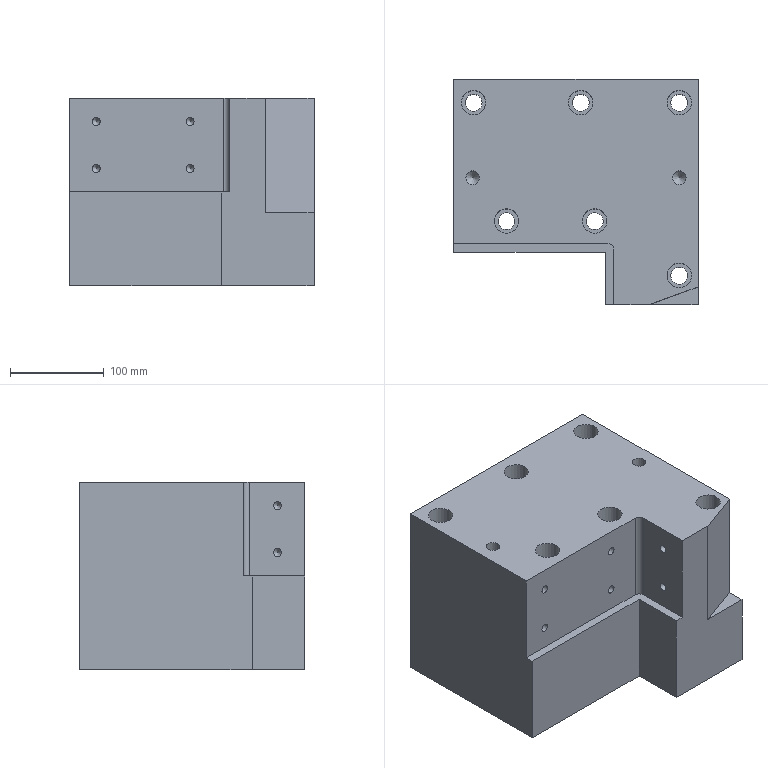Part | STEP file | lll_id4190_x_t | 1 solid | 48 faces | box 260 x 240 x 200 mm | volume 9818942 mm3 | cylinder 21 | plane 19 | cone 8 | commonest cylinder face diameters 8.506 x6 18.009 x6 26.008 x6 14.506 x2 12 x1
STEP:
#1=CARTESIAN_POINT('',(2885.753,309.047,34.253));
#2=VERTEX_POINT('',#1);
#3=CARTESIAN_POINT('',(2885.753,309.047,30.));
#4=DIRECTION('',(1.,0.,0.));
#5=DIRECTION('',(0.,0.,1.));
#6=AXIS2_PLACEMENT_3D('',#3,#4,#5);
#7=CIRCLE('',#6,4.253);
#8=EDGE_CURVE('',#2,#2,#7,.T.);
#9=ORIENTED_EDGE('',*,*,#8,.F.);
#10=EDGE_LOOP('',(#9));
#11=FACE_BOUND('',#10,.T.);
#12=CARTESIAN_POINT('',(2890.006,309.047,30.));
#13=VERTEX_POINT('',#12);
#14=VERTEX_LOOP('',#13);
#15=FACE_BOUND('',#14,.T.);
#16=CARTESIAN_POINT('',(2885.753,309.047,30.));
#17=DIRECTION('',(-1.,0.,0.));
#18=DIRECTION('',(0.,0.,-1.));
#19=AXIS2_PLACEMENT_3D('',#16,#17,#18);
#20=CONICAL_SURFACE('',#19,4.253,45.);
#21=ADVANCED_FACE('',(#11,#15),#20,.F.);
#22=CARTESIAN_POINT('',(2885.753,309.047,84.253));
#23=VERTEX_POINT('',#22);
#24=CARTESIAN_POINT('',(2885.753,309.047,80.));
#25=DIRECTION('',(1.,0.,0.));
#26=DIRECTION('',(0.,0.,1.));
#27=AXIS2_PLACEMENT_3D('',#24,#25,#26);
#28=CIRCLE('',#27,4.253);
#29=EDGE_CURVE('',#23,#23,#28,.T.);
#30=ORIENTED_EDGE('',*,*,#29,.F.);
#31=EDGE_LOOP('',(#30));
#32=FACE_BOUND('',#31,.T.);
#33=CARTESIAN_POINT('',(2890.006,309.047,80.));
#34=VERTEX_POINT('',#33);
#35=VERTEX_LOOP('',#34);
#36=FACE_BOUND('',#35,.T.);
#37=CARTESIAN_POINT('',(2885.753,309.047,80.));
#38=DIRECTION('',(-1.,0.,0.));
#39=DIRECTION('',(0.,0.,-1.));
#40=AXIS2_PLACEMENT_3D('',#37,#38,#39);
#41=CONICAL_SURFACE('',#40,4.253,45.);
#42=ADVANCED_FACE('',(#32,#36),#41,.F.);
#43=CARTESIAN_POINT('',(2703.,380.053,80.));
#44=VERTEX_POINT('',#43);
#45=VERTEX_LOOP('',#44);
#46=FACE_BOUND('',#45,.T.);
#47=CARTESIAN_POINT('',(2703.,375.8,75.747));
#48=VERTEX_POINT('',#47);
#49=CARTESIAN_POINT('',(2703.,375.8,80.));
#50=DIRECTION('',(0.,1.,0.));
#51=DIRECTION('',(0.,0.,-1.));
#52=AXIS2_PLACEMENT_3D('',#49,#50,#51);
#53=CIRCLE('',#52,4.253);
#54=EDGE_CURVE('',#48,#48,#53,.T.);
#55=ORIENTED_EDGE('',*,*,#54,.F.);
#56=EDGE_LOOP('',(#55));
#57=FACE_BOUND('',#56,.T.);
#58=CARTESIAN_POINT('',(2703.,375.8,80.));
#59=DIRECTION('',(0.,-1.,0.));
#60=DIRECTION('',(0.,0.,1.));
#61=AXIS2_PLACEMENT_3D('',#58,#59,#60);
#62=CONICAL_SURFACE('',#61,4.253,45.);
#63=ADVANCED_FACE('',(#46,#57),#62,.F.);
#64=CARTESIAN_POINT('',(2803.,380.053,80.));
#65=VERTEX_POINT('',#64);
#66=VERTEX_LOOP('',#65);
#67=FACE_BOUND('',#66,.T.);
#68=CARTESIAN_POINT('',(2803.,375.8,75.747));
#69=VERTEX_POINT('',#68);
#70=CARTESIAN_POINT('',(2803.,375.8,80.));
#71=DIRECTION('',(0.,1.,0.));
#72=DIRECTION('',(0.,0.,-1.));
#73=AXIS2_PLACEMENT_3D('',#70,#71,#72);
#74=CIRCLE('',#73,4.253);
#75=EDGE_CURVE('',#69,#69,#74,.T.);
#76=ORIENTED_EDGE('',*,*,#75,.F.);
#77=EDGE_LOOP('',(#76));
#78=FACE_BOUND('',#77,.T.);
#79=CARTESIAN_POINT('',(2803.,375.8,80.));
#80=DIRECTION('',(0.,-1.,0.));
#81=DIRECTION('',(0.,0.,1.));
#82=AXIS2_PLACEMENT_3D('',#79,#80,#81);
#83=CONICAL_SURFACE('',#82,4.253,45.);
#84=ADVANCED_FACE('',(#67,#78),#83,.F.);
#85=CARTESIAN_POINT('',(2703.,380.053,30.));
#86=VERTEX_POINT('',#85);
#87=VERTEX_LOOP('',#86);
#88=FACE_BOUND('',#87,.T.);
#89=CARTESIAN_POINT('',(2703.,375.8,25.747));
#90=VERTEX_POINT('',#89);
#91=CARTESIAN_POINT('',(2703.,375.8,30.));
#92=DIRECTION('',(0.,1.,0.));
#93=DIRECTION('',(0.,0.,-1.));
#94=AXIS2_PLACEMENT_3D('',#91,#92,#93);
#95=CIRCLE('',#94,4.253);
#96=EDGE_CURVE('',#90,#90,#95,.T.);
#97=ORIENTED_EDGE('',*,*,#96,.F.);
#98=EDGE_LOOP('',(#97));
#99=FACE_BOUND('',#98,.T.);
#100=CARTESIAN_POINT('',(2703.,375.8,30.));
#101=DIRECTION('',(0.,-1.,0.));
#102=DIRECTION('',(0.,0.,1.));
#103=AXIS2_PLACEMENT_3D('',#100,#101,#102);
#104=CONICAL_SURFACE('',#103,4.253,45.);
#105=ADVANCED_FACE('',(#88,#99),#104,.F.);
#106=CARTESIAN_POINT('',(2803.,380.053,30.));
#107=VERTEX_POINT('',#106);
#108=VERTEX_LOOP('',#107);
#109=FACE_BOUND('',#108,.T.);
#110=CARTESIAN_POINT('',(2803.,375.8,25.747));
#111=VERTEX_POINT('',#110);
#112=CARTESIAN_POINT('',(2803.,375.8,30.));
#113=DIRECTION('',(0.,1.,0.));
#114=DIRECTION('',(0.,0.,-1.));
#115=AXIS2_PLACEMENT_3D('',#112,#113,#114);
#116=CIRCLE('',#115,4.253);
#117=EDGE_CURVE('',#111,#111,#116,.T.);
#118=ORIENTED_EDGE('',*,*,#117,.F.);
#119=EDGE_LOOP('',(#118));
#120=FACE_BOUND('',#119,.T.);
#121=CARTESIAN_POINT('',(2803.,375.8,30.));
#122=DIRECTION('',(0.,-1.,0.));
#123=DIRECTION('',(0.,0.,1.));
#124=AXIS2_PLACEMENT_3D('',#121,#122,#123);
#125=CONICAL_SURFACE('',#124,4.253,45.);
#126=ADVANCED_FACE('',(#109,#120),#125,.F.);
#127=CARTESIAN_POINT('',(2924.005,495.047,-55.));
#128=VERTEX_POINT('',#127);
#129=CARTESIAN_POINT('',(2915.,495.047,-55.));
#130=DIRECTION('',(0.,0.,-1.));
#131=DIRECTION('',(1.,0.,0.));
#132=AXIS2_PLACEMENT_3D('',#129,#130,#131);
#133=CIRCLE('',#132,9.005);
#134=EDGE_CURVE('',#128,#128,#133,.T.);
#135=ORIENTED_EDGE('',*,*,#134,.T.);
#136=EDGE_LOOP('',(#135));
#137=FACE_BOUND('',#136,.T.);
#138=CARTESIAN_POINT('',(2901.996,495.047,-55.));
#139=VERTEX_POINT('',#138);
#140=CARTESIAN_POINT('',(2915.,495.047,-55.));
#141=DIRECTION('',(0.,0.,-1.));
#142=DIRECTION('',(-1.,0.,0.));
#143=AXIS2_PLACEMENT_3D('',#140,#141,#142);
#144=CIRCLE('',#143,13.004);
#145=EDGE_CURVE('',#139,#139,#144,.T.);
#146=ORIENTED_EDGE('',*,*,#145,.F.);
#147=EDGE_LOOP('',(#146));
#148=FACE_BOUND('',#147,.T.);
#149=CARTESIAN_POINT('',(2915.,495.047,-55.));
#150=DIRECTION('',(0.,0.,-1.));
#151=DIRECTION('',(1.,0.,0.));
#152=AXIS2_PLACEMENT_3D('',#149,#150,#151);
#153=PLANE('',#152);
#154=ADVANCED_FACE('',(#137,#148),#153,.F.);
#155=ORIENTED_EDGE('',*,*,#8,.T.);
#156=EDGE_LOOP('',(#155));
#157=FACE_BOUND('',#156,.T.);
#158=CARTESIAN_POINT('',(2845.,309.047,34.253));
#159=VERTEX_POINT('',#158);
#160=CARTESIAN_POINT('',(2845.,309.047,30.));
#161=DIRECTION('',(1.,0.,0.));
#162=DIRECTION('',(0.,0.,1.));
#163=AXIS2_PLACEMENT_3D('',#160,#161,#162);
#164=CIRCLE('',#163,4.253);
#165=EDGE_CURVE('',#159,#159,#164,.T.);
#166=ORIENTED_EDGE('',*,*,#165,.F.);
#167=EDGE_LOOP('',(#166));
#168=FACE_BOUND('',#167,.T.);
#169=CARTESIAN_POINT('',(2845.,309.047,30.));
#170=DIRECTION('',(1.,0.,0.));
#171=DIRECTION('',(0.,0.,1.));
#172=AXIS2_PLACEMENT_3D('',#169,#170,#171);
#173=CYLINDRICAL_SURFACE('',#172,4.253);
#174=ADVANCED_FACE('',(#157,#168),#173,.F.);
#175=ORIENTED_EDGE('',*,*,#29,.T.);
#176=EDGE_LOOP('',(#175));
#177=FACE_BOUND('',#176,.T.);
#178=CARTESIAN_POINT('',(2845.,309.047,84.253));
#179=VERTEX_POINT('',#178);
#180=CARTESIAN_POINT('',(2845.,309.047,80.));
#181=DIRECTION('',(1.,0.,0.));
#182=DIRECTION('',(0.,0.,1.));
#183=AXIS2_PLACEMENT_3D('',#180,#181,#182);
#184=CIRCLE('',#183,4.253);
#185=EDGE_CURVE('',#179,#179,#184,.T.);
#186=ORIENTED_EDGE('',*,*,#185,.F.);
#187=EDGE_LOOP('',(#186));
#188=FACE_BOUND('',#187,.T.);
#189=CARTESIAN_POINT('',(2845.,309.047,80.));
#190=DIRECTION('',(1.,0.,0.));
#191=DIRECTION('',(0.,0.,1.));
#192=AXIS2_PLACEMENT_3D('',#189,#190,#191);
#193=CYLINDRICAL_SURFACE('',#192,4.253);
#194=ADVANCED_FACE('',(#177,#188),#193,.F.);
#195=ORIENTED_EDGE('',*,*,#54,.T.);
#196=EDGE_LOOP('',(#195));
#197=FACE_BOUND('',#196,.T.);
#198=CARTESIAN_POINT('',(2698.747,345.047,80.));
#199=VERTEX_POINT('',#198);
#200=CARTESIAN_POINT('',(2703.,345.047,80.));
#201=DIRECTION('',(0.,1.,0.));
#202=DIRECTION('',(-1.,0.,0.));
#203=AXIS2_PLACEMENT_3D('',#200,#201,#202);
#204=CIRCLE('',#203,4.253);
#205=EDGE_CURVE('',#199,#199,#204,.T.);
#206=ORIENTED_EDGE('',*,*,#205,.F.);
#207=EDGE_LOOP('',(#206));
#208=FACE_BOUND('',#207,.T.);
#209=CARTESIAN_POINT('',(2703.,345.047,80.));
#210=DIRECTION('',(0.,1.,0.));
#211=DIRECTION('',(-1.,0.,0.));
#212=AXIS2_PLACEMENT_3D('',#209,#210,#211);
#213=CYLINDRICAL_SURFACE('',#212,4.253);
#214=ADVANCED_FACE('',(#197,#208),#213,.F.);
#215=ORIENTED_EDGE('',*,*,#75,.T.);
#216=EDGE_LOOP('',(#215));
#217=FACE_BOUND('',#216,.T.);
#218=CARTESIAN_POINT('',(2798.747,345.047,80.));
#219=VERTEX_POINT('',#218);
#220=CARTESIAN_POINT('',(2803.,345.047,80.));
#221=DIRECTION('',(0.,1.,0.));
#222=DIRECTION('',(-1.,0.,0.));
#223=AXIS2_PLACEMENT_3D('',#220,#221,#222);
#224=CIRCLE('',#223,4.253);
#225=EDGE_CURVE('',#219,#219,#224,.T.);
#226=ORIENTED_EDGE('',*,*,#225,.F.);
#227=EDGE_LOOP('',(#226));
#228=FACE_BOUND('',#227,.T.);
#229=CARTESIAN_POINT('',(2803.,345.047,80.));
#230=DIRECTION('',(0.,1.,0.));
#231=DIRECTION('',(-1.,0.,0.));
#232=AXIS2_PLACEMENT_3D('',#229,#230,#231);
#233=CYLINDRICAL_SURFACE('',#232,4.253);
#234=ADVANCED_FACE('',(#217,#228),#233,.F.);
#235=ORIENTED_EDGE('',*,*,#96,.T.);
#236=EDGE_LOOP('',(#235));
#237=FACE_BOUND('',#236,.T.);
#238=CARTESIAN_POINT('',(2698.747,345.047,30.));
#239=VERTEX_POINT('',#238);
#240=CARTESIAN_POINT('',(2703.,345.047,30.));
#241=DIRECTION('',(0.,1.,0.));
#242=DIRECTION('',(-1.,0.,0.));
#243=AXIS2_PLACEMENT_3D('',#240,#241,#242);
#244=CIRCLE('',#243,4.253);
#245=EDGE_CURVE('',#239,#239,#244,.T.);
#246=ORIENTED_EDGE('',*,*,#245,.F.);
#247=EDGE_LOOP('',(#246));
#248=FACE_BOUND('',#247,.T.);
#249=CARTESIAN_POINT('',(2703.,345.047,30.));
#250=DIRECTION('',(0.,1.,0.));
#251=DIRECTION('',(-1.,0.,0.));
#252=AXIS2_PLACEMENT_3D('',#249,#250,#251);
#253=CYLINDRICAL_SURFACE('',#252,4.253);
#254=ADVANCED_FACE('',(#237,#248),#253,.F.);
#255=ORIENTED_EDGE('',*,*,#117,.T.);
#256=EDGE_LOOP('',(#255));
#257=FACE_BOUND('',#256,.T.);
#258=CARTESIAN_POINT('',(2798.747,345.047,30.));
#259=VERTEX_POINT('',#258);
#260=CARTESIAN_POINT('',(2803.,345.047,30.));
#261=DIRECTION('',(0.,1.,0.));
#262=DIRECTION('',(-1.,0.,0.));
#263=AXIS2_PLACEMENT_3D('',#260,#261,#262);
#264=CIRCLE('',#263,4.253);
#265=EDGE_CURVE('',#259,#259,#264,.T.);
#266=ORIENTED_EDGE('',*,*,#265,.F.);
#267=EDGE_LOOP('',(#266));
#268=FACE_BOUND('',#267,.T.);
#269=CARTESIAN_POINT('',(2803.,345.047,30.));
#270=DIRECTION('',(0.,1.,0.));
#271=DIRECTION('',(-1.,0.,0.));
#272=AXIS2_PLACEMENT_3D('',#269,#270,#271);
#273=CYLINDRICAL_SURFACE('',#272,4.253);
#274=ADVANCED_FACE('',(#257,#268),#273,.F.);
#275=CARTESIAN_POINT('',(2845.,280.047,5.));
#276=VERTEX_POINT('',#275);
#277=CARTESIAN_POINT('',(2845.,339.047,5.));
#278=VERTEX_POINT('',#277);
#279=CARTESIAN_POINT('',(2845.,273.323,5.));
#280=DIRECTION('',(0.,1.,0.));
#281=VECTOR('',#280,1.);
#282=LINE('',#279,#281);
#283=EDGE_CURVE('',#276,#278,#282,.T.);
#284=ORIENTED_EDGE('',*,*,#283,.T.);
#285=CARTESIAN_POINT('',(2839.,345.047,5.));
#286=VERTEX_POINT('',#285);
#287=CARTESIAN_POINT('',(2839.,339.047,5.));
#288=DIRECTION('',(0.,0.,1.));
#289=DIRECTION('',(1.,0.,0.));
#290=AXIS2_PLACEMENT_3D('',#287,#288,#289);
#291=CIRCLE('',#290,6.);
#292=EDGE_CURVE('',#278,#286,#291,.T.);
#293=ORIENTED_EDGE('',*,*,#292,.T.);
#294=CARTESIAN_POINT('',(2675.,345.047,5.));
#295=VERTEX_POINT('',#294);
#296=CARTESIAN_POINT('',(2132.435,345.047,5.));
#297=DIRECTION('',(1.,0.,0.));
#298=VECTOR('',#297,1.);
#299=LINE('',#296,#298);
#300=EDGE_CURVE('',#295,#286,#299,.T.);
#301=ORIENTED_EDGE('',*,*,#300,.F.);
#302=CARTESIAN_POINT('',(2675.,336.047,5.));
#303=VERTEX_POINT('',#302);
#304=CARTESIAN_POINT('',(2675.,350.047,5.));
#305=DIRECTION('',(0.,1.,0.));
#306=VECTOR('',#305,1.);
#307=LINE('',#304,#306);
#308=EDGE_CURVE('',#303,#295,#307,.T.);
#309=ORIENTED_EDGE('',*,*,#308,.F.);
#310=CARTESIAN_POINT('',(2836.,336.047,5.));
#311=VERTEX_POINT('',#310);
#312=CARTESIAN_POINT('',(2132.435,336.047,5.));
#313=DIRECTION('',(-1.,0.,0.));
#314=VECTOR('',#313,1.);
#315=LINE('',#312,#314);
#316=EDGE_CURVE('',#311,#303,#315,.T.);
#317=ORIENTED_EDGE('',*,*,#316,.F.);
#318=CARTESIAN_POINT('',(2836.,280.047,5.));
#319=VERTEX_POINT('',#318);
#320=CARTESIAN_POINT('',(2836.,1.,5.));
#321=DIRECTION('',(0.,1.,0.));
#322=VECTOR('',#321,1.);
#323=LINE('',#320,#322);
#324=EDGE_CURVE('',#319,#311,#323,.T.);
#325=ORIENTED_EDGE('',*,*,#324,.F.);
#326=CARTESIAN_POINT('',(2132.435,280.047,5.));
#327=DIRECTION('',(1.,0.,0.));
#328=VECTOR('',#327,1.);
#329=LINE('',#326,#328);
#330=EDGE_CURVE('',#319,#276,#329,.T.);
#331=ORIENTED_EDGE('',*,*,#330,.T.);
#332=EDGE_LOOP('',(#284,#293,#301,#309,#317,#325,#331));
#333=FACE_OUTER_BOUND('',#332,.T.);
#334=CARTESIAN_POINT('',(2132.435,0.,5.));
#335=DIRECTION('',(0.,0.,1.));
#336=DIRECTION('',(1.,0.,0.));
#337=AXIS2_PLACEMENT_3D('',#334,#335,#336);
#338=PLANE('',#337);
#339=ADVANCED_FACE('',(#333),#338,.T.);
#340=CARTESIAN_POINT('',(2935.,280.047,-17.));
#341=VERTEX_POINT('',#340);
#342=CARTESIAN_POINT('',(2883.289,280.047,-17.));
#343=VERTEX_POINT('',#342);
#344=CARTESIAN_POINT('',(2655.,280.047,-17.));
#345=DIRECTION('',(-1.,0.,0.));
#346=VECTOR('',#345,1.);
#347=LINE('',#344,#346);
#348=EDGE_CURVE('',#341,#343,#347,.T.);
#349=ORIENTED_EDGE('',*,*,#348,.F.);
#350=CARTESIAN_POINT('',(2935.,298.868,-17.));
#351=VERTEX_POINT('',#350);
#352=CARTESIAN_POINT('',(2935.,365.047,-17.));
#353=DIRECTION('',(0.,-1.,0.));
#354=VECTOR('',#353,1.);
#355=LINE('',#352,#354);
#356=EDGE_CURVE('',#351,#341,#355,.T.);
#357=ORIENTED_EDGE('',*,*,#356,.F.);
#358=CARTESIAN_POINT('',(2927.313,296.07,-17.));
#359=DIRECTION('',(0.9397,0.342,0.));
#360=VECTOR('',#359,1.);
#361=LINE('',#358,#360);
#362=EDGE_CURVE('',#343,#351,#361,.T.);
#363=ORIENTED_EDGE('',*,*,#362,.F.);
#364=EDGE_LOOP('',(#349,#357,#363));
#365=FACE_OUTER_BOUND('',#364,.T.);
#366=CARTESIAN_POINT('',(2805.,365.047,-17.));
#367=DIRECTION('',(0.,0.,1.));
#368=DIRECTION('',(1.,0.,0.));
#369=AXIS2_PLACEMENT_3D('',#366,#367,#368);
#370=PLANE('',#369);
#371=ADVANCED_FACE('',(#365),#370,.T.);
#372=CARTESIAN_POINT('',(2695.,415.047,61.994));
#373=VERTEX_POINT('',#372);
#374=VERTEX_LOOP('',#373);
#375=FACE_BOUND('',#374,.T.);
#376=CARTESIAN_POINT('',(2702.253,415.047,69.247));
#377=VERTEX_POINT('',#376);
#378=CARTESIAN_POINT('',(2695.,415.047,69.247));
#379=DIRECTION('',(0.,0.,-1.));
#380=DIRECTION('',(1.,0.,0.));
#381=AXIS2_PLACEMENT_3D('',#378,#379,#380);
#382=CIRCLE('',#381,7.253);
#383=EDGE_CURVE('',#377,#377,#382,.T.);
#384=ORIENTED_EDGE('',*,*,#383,.F.);
#385=EDGE_LOOP('',(#384));
#386=FACE_BOUND('',#385,.T.);
#387=CARTESIAN_POINT('',(2695.,415.047,69.247));
#388=DIRECTION('',(0.,0.,1.));
#389=DIRECTION('',(-1.,0.,0.));
#390=AXIS2_PLACEMENT_3D('',#387,#388,#389);
#391=CONICAL_SURFACE('',#390,7.253,45.);
#392=ADVANCED_FACE('',(#375,#386),#391,.F.);
#393=CARTESIAN_POINT('',(2915.,415.047,61.994));
#394=VERTEX_POINT('',#393);
#395=VERTEX_LOOP('',#394);
#396=FACE_BOUND('',#395,.T.);
#397=CARTESIAN_POINT('',(2907.747,415.047,69.247));
#398=VERTEX_POINT('',#397);
#399=CARTESIAN_POINT('',(2915.,415.047,69.247));
#400=DIRECTION('',(0.,0.,-1.));
#401=DIRECTION('',(-1.,0.,0.));
#402=AXIS2_PLACEMENT_3D('',#399,#400,#401);
#403=CIRCLE('',#402,7.253);
#404=EDGE_CURVE('',#398,#398,#403,.T.);
#405=ORIENTED_EDGE('',*,*,#404,.F.);
#406=EDGE_LOOP('',(#405));
#407=FACE_BOUND('',#406,.T.);
#408=CARTESIAN_POINT('',(2915.,415.047,69.247));
#409=DIRECTION('',(0.,0.,1.));
#410=DIRECTION('',(1.,0.,0.));
#411=AXIS2_PLACEMENT_3D('',#408,#409,#410);
#412=CONICAL_SURFACE('',#411,7.253,45.);
#413=ADVANCED_FACE('',(#396,#407),#412,.F.);
#414=CARTESIAN_POINT('',(2924.005,311.047,-55.));
#415=VERTEX_POINT('',#414);
#416=CARTESIAN_POINT('',(2915.,311.047,-55.));
#417=DIRECTION('',(0.,0.,-1.));
#418=DIRECTION('',(1.,0.,0.));
#419=AXIS2_PLACEMENT_3D('',#416,#417,#418);
#420=CIRCLE('',#419,9.005);
#421=EDGE_CURVE('',#415,#415,#420,.T.);
#422=ORIENTED_EDGE('',*,*,#421,.T.);
#423=EDGE_LOOP('',(#422));
#424=FACE_BOUND('',#423,.T.);
#425=CARTESIAN_POINT('',(2901.996,311.047,-55.));
#426=VERTEX_POINT('',#425);
#427=CARTESIAN_POINT('',(2915.,311.047,-55.));
#428=DIRECTION('',(0.,0.,-1.));
#429=DIRECTION('',(-1.,0.,0.));
#430=AXIS2_PLACEMENT_3D('',#427,#428,#429);
#431=CIRCLE('',#430,13.004);
#432=EDGE_CURVE('',#426,#426,#431,.T.);
#433=ORIENTED_EDGE('',*,*,#432,.F.);
#434=EDGE_LOOP('',(#433));
#435=FACE_BOUND('',#434,.T.);
#436=CARTESIAN_POINT('',(2915.,311.047,-55.));
#437=DIRECTION('',(0.,0.,-1.));
#438=DIRECTION('',(1.,0.,0.));
#439=AXIS2_PLACEMENT_3D('',#436,#437,#438);
#440=PLANE('',#439);
#441=ADVANCED_FACE('',(#424,#435),#440,.F.);
#442=CARTESIAN_POINT('',(2819.005,495.047,-55.));
#443=VERTEX_POINT('',#442);
#444=CARTESIAN_POINT('',(2810.,495.047,-55.));
#445=DIRECTION('',(0.,0.,-1.));
#446=DIRECTION('',(1.,0.,0.));
#447=AXIS2_PLACEMENT_3D('',#444,#445,#446);
#448=CIRCLE('',#447,9.005);
#449=EDGE_CURVE('',#443,#443,#448,.T.);
#450=ORIENTED_EDGE('',*,*,#449,.T.);
#451=EDGE_LOOP('',(#450));
#452=FACE_BOUND('',#451,.T.);
#453=CARTESIAN_POINT('',(2796.996,495.047,-55.));
#454=VERTEX_POINT('',#453);
#455=CARTESIAN_POINT('',(2810.,495.047,-55.));
#456=DIRECTION('',(0.,0.,-1.));
#457=DIRECTION('',(-1.,0.,0.));
#458=AXIS2_PLACEMENT_3D('',#455,#456,#457);
#459=CIRCLE('',#458,13.004);
#460=EDGE_CURVE('',#454,#454,#459,.T.);
#461=ORIENTED_EDGE('',*,*,#460,.F.);
#462=EDGE_LOOP('',(#461));
#463=FACE_BOUND('',#462,.T.);
#464=CARTESIAN_POINT('',(2810.,495.047,-55.));
#465=DIRECTION('',(0.,0.,-1.));
#466=DIRECTION('',(1.,0.,0.));
#467=AXIS2_PLACEMENT_3D('',#464,#465,#466);
#468=PLANE('',#467);
#469=ADVANCED_FACE('',(#452,#463),#468,.F.);
#470=CARTESIAN_POINT('',(2705.005,495.047,-55.));
#471=VERTEX_POINT('',#470);
#472=CARTESIAN_POINT('',(2696.,495.047,-55.));
#473=DIRECTION('',(0.,0.,-1.));
#474=DIRECTION('',(1.,0.,0.));
#475=AXIS2_PLACEMENT_3D('',#472,#473,#474);
#476=CIRCLE('',#475,9.005);
#477=EDGE_CURVE('',#471,#471,#476,.T.);
#478=ORIENTED_EDGE('',*,*,#477,.T.);
#479=EDGE_LOOP('',(#478));
#480=FACE_BOUND('',#479,.T.);
#481=CARTESIAN_POINT('',(2682.996,495.047,-55.));
#482=VERTEX_POINT('',#481);
#483=CARTESIAN_POINT('',(2696.,495.047,-55.));
#484=DIRECTION('',(0.,0.,-1.));
#485=DIRECTION('',(-1.,0.,0.));
#486=AXIS2_PLACEMENT_3D('',#483,#484,#485);
#487=CIRCLE('',#486,13.004);
#488=EDGE_CURVE('',#482,#482,#487,.T.);
#489=ORIENTED_EDGE('',*,*,#488,.F.);
#490=EDGE_LOOP('',(#489));
#491=FACE_BOUND('',#490,.T.);
#492=CARTESIAN_POINT('',(2696.,495.047,-55.));
#493=DIRECTION('',(0.,0.,-1.));
#494=DIRECTION('',(1.,0.,0.));
#495=AXIS2_PLACEMENT_3D('',#492,#493,#494);
#496=PLANE('',#495);
#497=ADVANCED_FACE('',(#480,#491),#496,.F.);
#498=CARTESIAN_POINT('',(2834.005,369.047,-55.));
#499=VERTEX_POINT('',#498);
#500=CARTESIAN_POINT('',(2825.,369.047,-55.));
#501=DIRECTION('',(0.,0.,-1.));
#502=DIRECTION('',(1.,0.,0.));
#503=AXIS2_PLACEMENT_3D('',#500,#501,#502);
#504=CIRCLE('',#503,9.005);
#505=EDGE_CURVE('',#499,#499,#504,.T.);
#506=ORIENTED_EDGE('',*,*,#505,.T.);
#507=EDGE_LOOP('',(#506));
#508=FACE_BOUND('',#507,.T.);
#509=CARTESIAN_POINT('',(2811.996,369.047,-55.));
#510=VERTEX_POINT('',#509);
#511=CARTESIAN_POINT('',(2825.,369.047,-55.));
#512=DIRECTION('',(0.,0.,-1.));
#513=DIRECTION('',(-1.,0.,0.));
#514=AXIS2_PLACEMENT_3D('',#511,#512,#513);
#515=CIRCLE('',#514,13.004);
#516=EDGE_CURVE('',#510,#510,#515,.T.);
#517=ORIENTED_EDGE('',*,*,#516,.F.);
#518=EDGE_LOOP('',(#517));
#519=FACE_BOUND('',#518,.T.);
#520=CARTESIAN_POINT('',(2825.,369.047,-55.));
#521=DIRECTION('',(0.,0.,-1.));
#522=DIRECTION('',(1.,0.,0.));
#523=AXIS2_PLACEMENT_3D('',#520,#521,#522);
#524=PLANE('',#523);
#525=ADVANCED_FACE('',(#508,#519),#524,.F.);
#526=CARTESIAN_POINT('',(2675.,336.047,-95.));
#527=VERTEX_POINT('',#526);
#528=CARTESIAN_POINT('',(2675.,336.047,-65.));
#529=DIRECTION('',(0.,0.,-1.));
#530=VECTOR('',#529,1.);
#531=LINE('',#528,#530);
#532=EDGE_CURVE('',#303,#527,#531,.T.);
#533=ORIENTED_EDGE('',*,*,#532,.T.);
#534=CARTESIAN_POINT('',(2836.,336.047,-95.));
#535=VERTEX_POINT('',#534);
#536=CARTESIAN_POINT('',(2655.,336.047,-95.));
#537=DIRECTION('',(-1.,0.,0.));
#538=VECTOR('',#537,1.);
#539=LINE('',#536,#538);
#540=EDGE_CURVE('',#535,#527,#539,.T.);
#541=ORIENTED_EDGE('',*,*,#540,.F.);
#542=CARTESIAN_POINT('',(2836.,336.047,-650.));
#543=DIRECTION('',(0.,0.,-1.));
#544=VECTOR('',#543,1.);
#545=LINE('',#542,#544);
#546=EDGE_CURVE('',#311,#535,#545,.T.);
#547=ORIENTED_EDGE('',*,*,#546,.F.);
#548=ORIENTED_EDGE('',*,*,#316,.T.);
#549=EDGE_LOOP('',(#533,#541,#547,#548));
#550=FACE_OUTER_BOUND('',#549,.T.);
#551=CARTESIAN_POINT('',(-2196.249,336.047,-650.));
#552=DIRECTION('',(0.,-1.,0.));
#553=DIRECTION('',(0.,0.,1.));
#554=AXIS2_PLACEMENT_3D('',#551,#552,#553);
#555=PLANE('',#554);
#556=ADVANCED_FACE('',(#550),#555,.T.);
#557=ORIENTED_EDGE('',*,*,#546,.T.);
#558=CARTESIAN_POINT('',(2836.,280.047,-95.));
#559=VERTEX_POINT('',#558);
#560=CARTESIAN_POINT('',(2836.,1.,-95.));
#561=DIRECTION('',(0.,1.,0.));
#562=VECTOR('',#561,1.);
#563=LINE('',#560,#562);
#564=EDGE_CURVE('',#559,#535,#563,.T.);
#565=ORIENTED_EDGE('',*,*,#564,.F.);
#566=CARTESIAN_POINT('',(2836.,280.047,-650.));
#567=DIRECTION('',(0.,0.,1.));
#568=VECTOR('',#567,1.);
#569=LINE('',#566,#568);
#570=EDGE_CURVE('',#559,#319,#569,.T.);
#571=ORIENTED_EDGE('',*,*,#570,.T.);
#572=ORIENTED_EDGE('',*,*,#324,.T.);
#573=EDGE_LOOP('',(#557,#565,#571,#572));
#574=FACE_OUTER_BOUND('',#573,.T.);
#575=CARTESIAN_POINT('',(2836.,1.,-650.));
#576=DIRECTION('',(1.,0.,0.));
#577=DIRECTION('',(0.,0.,1.));
#578=AXIS2_PLACEMENT_3D('',#575,#576,#577);
#579=PLANE('',#578);
#580=ADVANCED_FACE('',(#574),#579,.F.);
#581=CARTESIAN_POINT('',(2924.005,495.047,-95.));
#582=VERTEX_POINT('',#581);
#583=CARTESIAN_POINT('',(2915.,495.047,-95.));
#584=DIRECTION('',(0.,0.,-1.));
#585=DIRECTION('',(1.,0.,0.));
#586=AXIS2_PLACEMENT_3D('',#583,#584,#585);
#587=CIRCLE('',#586,9.005);
#588=EDGE_CURVE('',#582,#582,#587,.T.);
#589=ORIENTED_EDGE('',*,*,#588,.T.);
#590=EDGE_LOOP('',(#589));
#591=FACE_BOUND('',#590,.T.);
#592=ORIENTED_EDGE('',*,*,#134,.F.);
#593=EDGE_LOOP('',(#592));
#594=FACE_BOUND('',#593,.T.);
#595=CARTESIAN_POINT('',(2915.,495.047,107.));
#596=DIRECTION('',(0.,0.,-1.));
#597=DIRECTION('',(-1.,0.,0.));
#598=AXIS2_PLACEMENT_3D('',#595,#596,#597);
#599=CYLINDRICAL_SURFACE('',#598,9.005);
#600=ADVANCED_FACE('',(#591,#594),#599,.F.);
#601=ORIENTED_EDGE('',*,*,#145,.T.);
#602=EDGE_LOOP('',(#601));
#603=FACE_BOUND('',#602,.T.);
#604=CARTESIAN_POINT('',(2901.996,495.047,105.));
#605=VERTEX_POINT('',#604);
#606=CARTESIAN_POINT('',(2915.,495.047,105.));
#607=DIRECTION('',(0.,0.,-1.));
#608=DIRECTION('',(-1.,0.,0.));
#609=AXIS2_PLACEMENT_3D('',#606,#607,#608);
#610=CIRCLE('',#609,13.004);
#611=EDGE_CURVE('',#605,#605,#610,.T.);
#612=ORIENTED_EDGE('',*,*,#611,.F.);
#613=EDGE_LOOP('',(#612));
#614=FACE_BOUND('',#613,.T.);
#615=CARTESIAN_POINT('',(2915.,495.047,105.));
#616=DIRECTION('',(0.,0.,-1.));
#617=DIRECTION('',(-1.,0.,0.));
#618=AXIS2_PLACEMENT_3D('',#615,#616,#617);
#619=CYLINDRICAL_SURFACE('',#618,13.004);
#620=ADVANCED_FACE('',(#603,#614),#619,.F.);
#621=ORIENTED_EDGE('',*,*,#362,.T.);
#622=CARTESIAN_POINT('',(2935.,298.868,105.));
#623=VERTEX_POINT('',#622);
#624=CARTESIAN_POINT('',(2935.,298.868,-80.));
#625=DIRECTION('',(0.,0.,1.));
#626=VECTOR('',#625,1.);
#627=LINE('',#624,#626);
#628=EDGE_CURVE('',#351,#623,#627,.T.);
#629=ORIENTED_EDGE('',*,*,#628,.T.);
#630=CARTESIAN_POINT('',(2883.289,280.047,105.));
#631=VERTEX_POINT('',#630);
#632=CARTESIAN_POINT('',(2677.687,205.214,105.));
#633=DIRECTION('',(-0.9397,-0.342,0.));
#634=VECTOR('',#633,1.);
#635=LINE('',#632,#634);
#636=EDGE_CURVE('',#623,#631,#635,.T.);
#637=ORIENTED_EDGE('',*,*,#636,.T.);
#638=CARTESIAN_POINT('',(2883.289,280.047,-80.));
#639=DIRECTION('',(0.,0.,-1.));
#640=VECTOR('',#639,1.);
#641=LINE('',#638,#640);
#642=EDGE_CURVE('',#631,#343,#641,.T.);
#643=ORIENTED_EDGE('',*,*,#642,.T.);
#644=EDGE_LOOP('',(#621,#629,#637,#643));
#645=FACE_OUTER_BOUND('',#644,.T.);
#646=CARTESIAN_POINT('',(2927.313,296.07,-80.));
#647=DIRECTION('',(0.342,-0.9397,0.));
#648=DIRECTION('',(0.,0.,-1.));
#649=AXIS2_PLACEMENT_3D('',#646,#647,#648);
#650=PLANE('',#649);
#651=ADVANCED_FACE('',(#645),#650,.T.);
#652=ORIENTED_EDGE('',*,*,#348,.T.);
#653=ORIENTED_EDGE('',*,*,#642,.F.);
#654=CARTESIAN_POINT('',(2845.,280.047,105.));
#655=VERTEX_POINT('',#654);
#656=CARTESIAN_POINT('',(2655.,280.047,105.));
#657=DIRECTION('',(-1.,0.,0.));
#658=VECTOR('',#657,1.);
#659=LINE('',#656,#658);
#660=EDGE_CURVE('',#631,#655,#659,.T.);
#661=ORIENTED_EDGE('',*,*,#660,.T.);
#662=CARTESIAN_POINT('',(2845.,280.047,171.231));
#663=DIRECTION('',(0.,0.,1.));
#664=VECTOR('',#663,1.);
#665=LINE('',#662,#664);
#666=EDGE_CURVE('',#276,#655,#665,.T.);
#667=ORIENTED_EDGE('',*,*,#666,.F.);
#668=ORIENTED_EDGE('',*,*,#330,.F.);
#669=ORIENTED_EDGE('',*,*,#570,.F.);
#670=CARTESIAN_POINT('',(2935.,280.047,-95.));
#671=VERTEX_POINT('',#670);
#672=CARTESIAN_POINT('',(2655.,280.047,-95.));
#673=DIRECTION('',(-1.,0.,0.));
#674=VECTOR('',#673,1.);
#675=LINE('',#672,#674);
#676=EDGE_CURVE('',#671,#559,#675,.T.);
#677=ORIENTED_EDGE('',*,*,#676,.F.);
#678=CARTESIAN_POINT('',(2935.,280.047,-65.));
#679=DIRECTION('',(0.,0.,-1.));
#680=VECTOR('',#679,1.);
#681=LINE('',#678,#680);
#682=EDGE_CURVE('',#341,#671,#681,.T.);
#683=ORIENTED_EDGE('',*,*,#682,.F.);
#684=EDGE_LOOP('',(#652,#653,#661,#667,#668,#669,#677,#683));
#685=FACE_OUTER_BOUND('',#684,.T.);
#686=CARTESIAN_POINT('',(2655.,280.047,-65.));
#687=DIRECTION('',(0.,1.,0.));
#688=DIRECTION('',(0.,0.,-1.));
#689=AXIS2_PLACEMENT_3D('',#686,#687,#688);
#690=PLANE('',#689);
#691=ADVANCED_FACE('',(#685),#690,.F.);
#692=ORIENTED_EDGE('',*,*,#185,.T.);
#693=EDGE_LOOP('',(#692));
#694=FACE_BOUND('',#693,.T.);
#695=ORIENTED_EDGE('',*,*,#165,.T.);
#696=EDGE_LOOP('',(#695));
#697=FACE_BOUND('',#696,.T.);
#698=CARTESIAN_POINT('',(2845.,339.047,105.));
#699=VERTEX_POINT('',#698);
#700=CARTESIAN_POINT('',(2845.,267.547,105.));
#701=DIRECTION('',(0.,1.,0.));
#702=VECTOR('',#701,1.);
#703=LINE('',#700,#702);
#704=EDGE_CURVE('',#655,#699,#703,.T.);
#705=ORIENTED_EDGE('',*,*,#704,.T.);
#706=CARTESIAN_POINT('',(2845.,339.047,5.));
#707=DIRECTION('',(0.,0.,-1.));
#708=VECTOR('',#707,1.);
#709=LINE('',#706,#708);
#710=EDGE_CURVE('',#699,#278,#709,.T.);
#711=ORIENTED_EDGE('',*,*,#710,.T.);
#712=ORIENTED_EDGE('',*,*,#283,.F.);
#713=ORIENTED_EDGE('',*,*,#666,.T.);
#714=EDGE_LOOP('',(#705,#711,#712,#713));
#715=FACE_BOUND('',#714,.T.);
#716=CARTESIAN_POINT('',(2845.,273.323,171.231));
#717=DIRECTION('',(1.,0.,0.));
#718=DIRECTION('',(0.,0.,1.));
#719=AXIS2_PLACEMENT_3D('',#716,#717,#718);
#720=PLANE('',#719);
#721=ADVANCED_FACE('',(#694,#697,#715),#720,.F.);
#722=ORIENTED_EDGE('',*,*,#265,.T.);
#723=EDGE_LOOP('',(#722));
#724=FACE_BOUND('',#723,.T.);
#725=ORIENTED_EDGE('',*,*,#245,.T.);
#726=EDGE_LOOP('',(#725));
#727=FACE_BOUND('',#726,.T.);
#728=ORIENTED_EDGE('',*,*,#225,.T.);
#729=EDGE_LOOP('',(#728));
#730=FACE_BOUND('',#729,.T.);
#731=ORIENTED_EDGE('',*,*,#205,.T.);
#732=EDGE_LOOP('',(#731));
#733=FACE_BOUND('',#732,.T.);
#734=ORIENTED_EDGE('',*,*,#300,.T.);
#735=CARTESIAN_POINT('',(2839.,345.047,105.));
#736=VERTEX_POINT('',#735);
#737=CARTESIAN_POINT('',(2839.,345.047,105.));
#738=DIRECTION('',(0.,0.,1.));
#739=VECTOR('',#738,1.);
#740=LINE('',#737,#739);
#741=EDGE_CURVE('',#286,#736,#740,.T.);
#742=ORIENTED_EDGE('',*,*,#741,.T.);
#743=CARTESIAN_POINT('',(2675.,345.047,105.));
#744=VERTEX_POINT('',#743);
#745=CARTESIAN_POINT('',(2655.,345.047,105.));
#746=DIRECTION('',(-1.,0.,0.));
#747=VECTOR('',#746,1.);
#748=LINE('',#745,#747);
#749=EDGE_CURVE('',#736,#744,#748,.T.);
#750=ORIENTED_EDGE('',*,*,#749,.T.);
#751=CARTESIAN_POINT('',(2675.,345.047,170.851));
#752=DIRECTION('',(0.,0.,-1.));
#753=VECTOR('',#752,1.);
#754=LINE('',#751,#753);
#755=EDGE_CURVE('',#744,#295,#754,.T.);
#756=ORIENTED_EDGE('',*,*,#755,.T.);
#757=EDGE_LOOP('',(#734,#742,#750,#756));
#758=FACE_BOUND('',#757,.T.);
#759=CARTESIAN_POINT('',(2685.,345.047,170.851));
#760=DIRECTION('',(0.,1.,0.));
#761=DIRECTION('',(0.,0.,-1.));
#762=AXIS2_PLACEMENT_3D('',#759,#760,#761);
#763=PLANE('',#762);
#764=ADVANCED_FACE('',(#724,#727,#730,#733,#758),#763,.F.);
#765=CARTESIAN_POINT('',(2675.,520.047,-95.));
#766=VERTEX_POINT('',#765);
#767=CARTESIAN_POINT('',(2675.,520.047,105.));
#768=VERTEX_POINT('',#767);
#769=CARTESIAN_POINT('',(2675.,520.047,-65.));
#770=DIRECTION('',(0.,0.,1.));
#771=VECTOR('',#770,1.);
#772=LINE('',#769,#771);
#773=EDGE_CURVE('',#766,#768,#772,.T.);
#774=ORIENTED_EDGE('',*,*,#773,.F.);
#775=CARTESIAN_POINT('',(2675.,350.047,-95.));
#776=DIRECTION('',(0.,1.,0.));
#777=VECTOR('',#776,1.);
#778=LINE('',#775,#777);
#779=EDGE_CURVE('',#527,#766,#778,.T.);
#780=ORIENTED_EDGE('',*,*,#779,.F.);
#781=ORIENTED_EDGE('',*,*,#532,.F.);
#782=ORIENTED_EDGE('',*,*,#308,.T.);
#783=ORIENTED_EDGE('',*,*,#755,.F.);
#784=CARTESIAN_POINT('',(2675.,267.547,105.));
#785=DIRECTION('',(0.,1.,0.));
#786=VECTOR('',#785,1.);
#787=LINE('',#784,#786);
#788=EDGE_CURVE('',#744,#768,#787,.T.);
#789=ORIENTED_EDGE('',*,*,#788,.T.);
#790=EDGE_LOOP('',(#774,#780,#781,#782,#783,#789));
#791=FACE_OUTER_BOUND('',#790,.T.);
#792=CARTESIAN_POINT('',(2675.,350.047,-65.));
#793=DIRECTION('',(1.,0.,0.));
#794=DIRECTION('',(0.,0.,1.));
#795=AXIS2_PLACEMENT_3D('',#792,#793,#794);
#796=PLANE('',#795);
#797=ADVANCED_FACE('',(#791),#796,.F.);
#798=CARTESIAN_POINT('',(2935.,520.047,-95.));
#799=VERTEX_POINT('',#798);
#800=CARTESIAN_POINT('',(2935.,520.047,105.));
#801=VERTEX_POINT('',#800);
#802=CARTESIAN_POINT('',(2935.,520.047,-80.));
#803=DIRECTION('',(0.,0.,1.));
#804=VECTOR('',#803,1.);
#805=LINE('',#802,#804);
#806=EDGE_CURVE('',#799,#801,#805,.T.);
#807=ORIENTED_EDGE('',*,*,#806,.F.);
#808=CARTESIAN_POINT('',(2655.,520.047,-95.));
#809=DIRECTION('',(-1.,0.,0.));
#810=VECTOR('',#809,1.);
#811=LINE('',#808,#810);
#812=EDGE_CURVE('',#799,#766,#811,.T.);
#813=ORIENTED_EDGE('',*,*,#812,.T.);
#814=ORIENTED_EDGE('',*,*,#773,.T.);
#815=CARTESIAN_POINT('',(2655.,520.047,105.));
#816=DIRECTION('',(1.,0.,0.));
#817=VECTOR('',#816,1.);
#818=LINE('',#815,#817);
#819=EDGE_CURVE('',#768,#801,#818,.T.);
#820=ORIENTED_EDGE('',*,*,#819,.T.);
#821=EDGE_LOOP('',(#807,#813,#814,#820));
#822=FACE_OUTER_BOUND('',#821,.T.);
#823=CARTESIAN_POINT('',(2655.,520.047,-80.));
#824=DIRECTION('',(0.,1.,0.));
#825=DIRECTION('',(0.,0.,-1.));
#826=AXIS2_PLACEMENT_3D('',#823,#824,#825);
#827=PLANE('',#826);
#828=ADVANCED_FACE('',(#822),#827,.T.);
#829=ORIENTED_EDGE('',*,*,#356,.T.);
#830=ORIENTED_EDGE('',*,*,#682,.T.);
#831=CARTESIAN_POINT('',(2935.,267.547,-95.));
#832=DIRECTION('',(0.,1.,0.));
#833=VECTOR('',#832,1.);
#834=LINE('',#831,#833);
#835=EDGE_CURVE('',#671,#799,#834,.T.);
#836=ORIENTED_EDGE('',*,*,#835,.T.);
#837=ORIENTED_EDGE('',*,*,#806,.T.);
#838=CARTESIAN_POINT('',(2935.,267.547,105.));
#839=DIRECTION('',(0.,-1.,0.));
#840=VECTOR('',#839,1.);
#841=LINE('',#838,#840);
#842=EDGE_CURVE('',#801,#623,#841,.T.);
#843=ORIENTED_EDGE('',*,*,#842,.T.);
#844=ORIENTED_EDGE('',*,*,#628,.F.);
#845=EDGE_LOOP('',(#829,#830,#836,#837,#843,#844));
#846=FACE_OUTER_BOUND('',#845,.T.);
#847=CARTESIAN_POINT('',(2935.,267.547,-80.));
#848=DIRECTION('',(1.,0.,0.));
#849=DIRECTION('',(0.,0.,1.));
#850=AXIS2_PLACEMENT_3D('',#847,#848,#849);
#851=PLANE('',#850);
#852=ADVANCED_FACE('',(#846),#851,.T.);
#853=CARTESIAN_POINT('',(2687.747,415.047,105.));
#854=VERTEX_POINT('',#853);
#855=CARTESIAN_POINT('',(2695.,415.047,105.));
#856=DIRECTION('',(0.,0.,1.));
#857=DIRECTION('',(-1.,0.,0.));
#858=AXIS2_PLACEMENT_3D('',#855,#856,#857);
#859=CIRCLE('',#858,7.253);
#860=EDGE_CURVE('',#854,#854,#859,.T.);
#861=ORIENTED_EDGE('',*,*,#860,.T.);
#862=EDGE_LOOP('',(#861));
#863=FACE_BOUND('',#862,.T.);
#864=ORIENTED_EDGE('',*,*,#383,.T.);
#865=EDGE_LOOP('',(#864));
#866=FACE_BOUND('',#865,.T.);
#867=CARTESIAN_POINT('',(2695.,415.047,107.));
#868=DIRECTION('',(0.,0.,-1.));
#869=DIRECTION('',(-1.,0.,0.));
#870=AXIS2_PLACEMENT_3D('',#867,#868,#869);
#871=CYLINDRICAL_SURFACE('',#870,7.253);
#872=ADVANCED_FACE('',(#863,#866),#871,.F.);
#873=CARTESIAN_POINT('',(2922.253,415.047,105.));
#874=VERTEX_POINT('',#873);
#875=CARTESIAN_POINT('',(2915.,415.047,105.));
#876=DIRECTION('',(0.,0.,1.));
#877=DIRECTION('',(1.,0.,0.));
#878=AXIS2_PLACEMENT_3D('',#875,#876,#877);
#879=CIRCLE('',#878,7.253);
#880=EDGE_CURVE('',#874,#874,#879,.T.);
#881=ORIENTED_EDGE('',*,*,#880,.T.);
#882=EDGE_LOOP('',(#881));
#883=FACE_BOUND('',#882,.T.);
#884=ORIENTED_EDGE('',*,*,#404,.T.);
#885=EDGE_LOOP('',(#884));
#886=FACE_BOUND('',#885,.T.);
#887=CARTESIAN_POINT('',(2915.,415.047,107.));
#888=DIRECTION('',(0.,0.,-1.));
#889=DIRECTION('',(1.,0.,0.));
#890=AXIS2_PLACEMENT_3D('',#887,#888,#889);
#891=CYLINDRICAL_SURFACE('',#890,7.253);
#892=ADVANCED_FACE('',(#883,#886),#891,.F.);
#893=ORIENTED_EDGE('',*,*,#432,.T.);
#894=EDGE_LOOP('',(#893));
#895=FACE_BOUND('',#894,.T.);
#896=CARTESIAN_POINT('',(2928.004,311.047,105.));
#897=VERTEX_POINT('',#896);
#898=CARTESIAN_POINT('',(2915.,311.047,105.));
#899=DIRECTION('',(0.,0.,1.));
#900=DIRECTION('',(1.,0.,0.));
#901=AXIS2_PLACEMENT_3D('',#898,#899,#900);
#902=CIRCLE('',#901,13.004);
#903=EDGE_CURVE('',#897,#897,#902,.T.);
#904=ORIENTED_EDGE('',*,*,#903,.T.);
#905=EDGE_LOOP('',(#904));
#906=FACE_BOUND('',#905,.T.);
#907=CARTESIAN_POINT('',(2915.,311.047,105.));
#908=DIRECTION('',(0.,0.,-1.));
#909=DIRECTION('',(-1.,0.,0.));
#910=AXIS2_PLACEMENT_3D('',#907,#908,#909);
#911=CYLINDRICAL_SURFACE('',#910,13.004);
#912=ADVANCED_FACE('',(#895,#906),#911,.F.);
#913=ORIENTED_EDGE('',*,*,#460,.T.);
#914=EDGE_LOOP('',(#913));
#915=FACE_BOUND('',#914,.T.);
#916=CARTESIAN_POINT('',(2823.004,495.047,105.));
#917=VERTEX_POINT('',#916);
#918=CARTESIAN_POINT('',(2810.,495.047,105.));
#919=DIRECTION('',(0.,0.,1.));
#920=DIRECTION('',(1.,0.,0.));
#921=AXIS2_PLACEMENT_3D('',#918,#919,#920);
#922=CIRCLE('',#921,13.004);
#923=EDGE_CURVE('',#917,#917,#922,.T.);
#924=ORIENTED_EDGE('',*,*,#923,.T.);
#925=EDGE_LOOP('',(#924));
#926=FACE_BOUND('',#925,.T.);
#927=CARTESIAN_POINT('',(2810.,495.047,105.));
#928=DIRECTION('',(0.,0.,-1.));
#929=DIRECTION('',(-1.,0.,0.));
#930=AXIS2_PLACEMENT_3D('',#927,#928,#929);
#931=CYLINDRICAL_SURFACE('',#930,13.004);
#932=ADVANCED_FACE('',(#915,#926),#931,.F.);
#933=ORIENTED_EDGE('',*,*,#488,.T.);
#934=EDGE_LOOP('',(#933));
#935=FACE_BOUND('',#934,.T.);
#936=CARTESIAN_POINT('',(2709.004,495.047,105.));
#937=VERTEX_POINT('',#936);
#938=CARTESIAN_POINT('',(2696.,495.047,105.));
#939=DIRECTION('',(0.,0.,1.));
#940=DIRECTION('',(1.,0.,0.));
#941=AXIS2_PLACEMENT_3D('',#938,#939,#940);
#942=CIRCLE('',#941,13.004);
#943=EDGE_CURVE('',#937,#937,#942,.T.);
#944=ORIENTED_EDGE('',*,*,#943,.T.);
#945=EDGE_LOOP('',(#944));
#946=FACE_BOUND('',#945,.T.);
#947=CARTESIAN_POINT('',(2696.,495.047,105.));
#948=DIRECTION('',(0.,0.,-1.));
#949=DIRECTION('',(-1.,0.,0.));
#950=AXIS2_PLACEMENT_3D('',#947,#948,#949);
#951=CYLINDRICAL_SURFACE('',#950,13.004);
#952=ADVANCED_FACE('',(#935,#946),#951,.F.);
#953=ORIENTED_EDGE('',*,*,#516,.T.);
#954=EDGE_LOOP('',(#953));
#955=FACE_BOUND('',#954,.T.);
#956=CARTESIAN_POINT('',(2838.004,369.047,105.));
#957=VERTEX_POINT('',#956);
#958=CARTESIAN_POINT('',(2825.,369.047,105.));
#959=DIRECTION('',(0.,0.,1.));
#960=DIRECTION('',(1.,0.,0.));
#961=AXIS2_PLACEMENT_3D('',#958,#959,#960);
#962=CIRCLE('',#961,13.004);
#963=EDGE_CURVE('',#957,#957,#962,.T.);
#964=ORIENTED_EDGE('',*,*,#963,.T.);
#965=EDGE_LOOP('',(#964));
#966=FACE_BOUND('',#965,.T.);
#967=CARTESIAN_POINT('',(2825.,369.047,105.));
#968=DIRECTION('',(0.,0.,-1.));
#969=DIRECTION('',(-1.,0.,0.));
#970=AXIS2_PLACEMENT_3D('',#967,#968,#969);
#971=CYLINDRICAL_SURFACE('',#970,13.004);
#972=ADVANCED_FACE('',(#955,#966),#971,.F.);
#973=CARTESIAN_POINT('',(2744.004,369.047,105.));
#974=VERTEX_POINT('',#973);
#975=CARTESIAN_POINT('',(2731.,369.047,105.));
#976=DIRECTION('',(0.,0.,1.));
#977=DIRECTION('',(1.,0.,0.));
#978=AXIS2_PLACEMENT_3D('',#975,#976,#977);
#979=CIRCLE('',#978,13.004);
#980=EDGE_CURVE('',#974,#974,#979,.T.);
#981=ORIENTED_EDGE('',*,*,#980,.F.);
#982=EDGE_LOOP('',(#981));
#983=FACE_BOUND('',#982,.T.);
#984=ORIENTED_EDGE('',*,*,#963,.F.);
#985=EDGE_LOOP('',(#984));
#986=FACE_BOUND('',#985,.T.);
#987=ORIENTED_EDGE('',*,*,#943,.F.);
#988=EDGE_LOOP('',(#987));
#989=FACE_BOUND('',#988,.T.);
#990=ORIENTED_EDGE('',*,*,#923,.F.);
#991=EDGE_LOOP('',(#990));
#992=FACE_BOUND('',#991,.T.);
#993=ORIENTED_EDGE('',*,*,#903,.F.);
#994=EDGE_LOOP('',(#993));
#995=FACE_BOUND('',#994,.T.);
#996=ORIENTED_EDGE('',*,*,#880,.F.);
#997=EDGE_LOOP('',(#996));
#998=FACE_BOUND('',#997,.T.);
#999=ORIENTED_EDGE('',*,*,#860,.F.);
#1000=EDGE_LOOP('',(#999));
#1001=FACE_BOUND('',#1000,.T.);
#1002=ORIENTED_EDGE('',*,*,#842,.F.);
#1003=ORIENTED_EDGE('',*,*,#819,.F.);
#1004=ORIENTED_EDGE('',*,*,#788,.F.);
#1005=ORIENTED_EDGE('',*,*,#749,.F.);
#1006=CARTESIAN_POINT('',(2839.,339.047,105.));
#1007=DIRECTION('',(0.,0.,-1.));
#1008=DIRECTION('',(1.,0.,0.));
#1009=AXIS2_PLACEMENT_3D('',#1006,#1007,#1008);
#1010=CIRCLE('',#1009,6.);
#1011=EDGE_CURVE('',#736,#699,#1010,.T.);
#1012=ORIENTED_EDGE('',*,*,#1011,.T.);
#1013=ORIENTED_EDGE('',*,*,#704,.F.);
#1014=ORIENTED_EDGE('',*,*,#660,.F.);
#1015=ORIENTED_EDGE('',*,*,#636,.F.);
#1016=EDGE_LOOP('',(#1002,#1003,#1004,#1005,#1012,#1013,#1014,#1015));
#1017=FACE_BOUND('',#1016,.T.);
#1018=ORIENTED_EDGE('',*,*,#611,.T.);
#1019=EDGE_LOOP('',(#1018));
#1020=FACE_BOUND('',#1019,.T.);
#1021=CARTESIAN_POINT('',(2655.,267.547,105.));
#1022=DIRECTION('',(0.,0.,1.));
#1023=DIRECTION('',(-1.,0.,0.));
#1024=AXIS2_PLACEMENT_3D('',#1021,#1022,#1023);
#1025=PLANE('',#1024);
#1026=ADVANCED_FACE('',(#983,#986,#989,#992,#995,#998,#1001,#1017,#1020),#1025,.T.);
#1027=CARTESIAN_POINT('',(2905.995,311.047,-95.));
#1028=VERTEX_POINT('',#1027);
#1029=CARTESIAN_POINT('',(2915.,311.047,-95.));
#1030=DIRECTION('',(0.,0.,-1.));
#1031=DIRECTION('',(-1.,0.,0.));
#1032=AXIS2_PLACEMENT_3D('',#1029,#1030,#1031);
#1033=CIRCLE('',#1032,9.005);
#1034=EDGE_CURVE('',#1028,#1028,#1033,.T.);
#1035=ORIENTED_EDGE('',*,*,#1034,.T.);
#1036=EDGE_LOOP('',(#1035));
#1037=FACE_BOUND('',#1036,.T.);
#1038=ORIENTED_EDGE('',*,*,#421,.F.);
#1039=EDGE_LOOP('',(#1038));
#1040=FACE_BOUND('',#1039,.T.);
#1041=CARTESIAN_POINT('',(2915.,311.047,107.));
#1042=DIRECTION('',(0.,0.,-1.));
#1043=DIRECTION('',(-1.,0.,0.));
#1044=AXIS2_PLACEMENT_3D('',#1041,#1042,#1043);
#1045=CYLINDRICAL_SURFACE('',#1044,9.005);
#1046=ADVANCED_FACE('',(#1037,#1040),#1045,.F.);
#1047=CARTESIAN_POINT('',(2800.995,495.047,-95.));
#1048=VERTEX_POINT('',#1047);
#1049=CARTESIAN_POINT('',(2810.,495.047,-95.));
#1050=DIRECTION('',(0.,0.,-1.));
#1051=DIRECTION('',(-1.,0.,0.));
#1052=AXIS2_PLACEMENT_3D('',#1049,#1050,#1051);
#1053=CIRCLE('',#1052,9.005);
#1054=EDGE_CURVE('',#1048,#1048,#1053,.T.);
#1055=ORIENTED_EDGE('',*,*,#1054,.T.);
#1056=EDGE_LOOP('',(#1055));
#1057=FACE_BOUND('',#1056,.T.);
#1058=ORIENTED_EDGE('',*,*,#449,.F.);
#1059=EDGE_LOOP('',(#1058));
#1060=FACE_BOUND('',#1059,.T.);
#1061=CARTESIAN_POINT('',(2810.,495.047,107.));
#1062=DIRECTION('',(0.,0.,-1.));
#1063=DIRECTION('',(-1.,0.,0.));
#1064=AXIS2_PLACEMENT_3D('',#1061,#1062,#1063);
#1065=CYLINDRICAL_SURFACE('',#1064,9.005);
#1066=ADVANCED_FACE('',(#1057,#1060),#1065,.F.);
#1067=CARTESIAN_POINT('',(2686.995,495.047,-95.));
#1068=VERTEX_POINT('',#1067);
#1069=CARTESIAN_POINT('',(2696.,495.047,-95.));
#1070=DIRECTION('',(0.,0.,-1.));
#1071=DIRECTION('',(-1.,0.,0.));
#1072=AXIS2_PLACEMENT_3D('',#1069,#1070,#1071);
#1073=CIRCLE('',#1072,9.005);
#1074=EDGE_CURVE('',#1068,#1068,#1073,.T.);
#1075=ORIENTED_EDGE('',*,*,#1074,.T.);
#1076=EDGE_LOOP('',(#1075));
#1077=FACE_BOUND('',#1076,.T.);
#1078=ORIENTED_EDGE('',*,*,#477,.F.);
#1079=EDGE_LOOP('',(#1078));
#1080=FACE_BOUND('',#1079,.T.);
#1081=CARTESIAN_POINT('',(2696.,495.047,107.));
#1082=DIRECTION('',(0.,0.,-1.));
#1083=DIRECTION('',(-1.,0.,0.));
#1084=AXIS2_PLACEMENT_3D('',#1081,#1082,#1083);
#1085=CYLINDRICAL_SURFACE('',#1084,9.005);
#1086=ADVANCED_FACE('',(#1077,#1080),#1085,.F.);
#1087=CARTESIAN_POINT('',(2815.995,369.047,-95.));
#1088=VERTEX_POINT('',#1087);
#1089=CARTESIAN_POINT('',(2825.,369.047,-95.));
#1090=DIRECTION('',(0.,0.,-1.));
#1091=DIRECTION('',(-1.,0.,0.));
#1092=AXIS2_PLACEMENT_3D('',#1089,#1090,#1091);
#1093=CIRCLE('',#1092,9.005);
#1094=EDGE_CURVE('',#1088,#1088,#1093,.T.);
#1095=ORIENTED_EDGE('',*,*,#1094,.T.);
#1096=EDGE_LOOP('',(#1095));
#1097=FACE_BOUND('',#1096,.T.);
#1098=ORIENTED_EDGE('',*,*,#505,.F.);
#1099=EDGE_LOOP('',(#1098));
#1100=FACE_BOUND('',#1099,.T.);
#1101=CARTESIAN_POINT('',(2825.,369.047,107.));
#1102=DIRECTION('',(0.,0.,-1.));
#1103=DIRECTION('',(-1.,0.,0.));
#1104=AXIS2_PLACEMENT_3D('',#1101,#1102,#1103);
#1105=CYLINDRICAL_SURFACE('',#1104,9.005);
#1106=ADVANCED_FACE('',(#1097,#1100),#1105,.F.);
#1107=CARTESIAN_POINT('',(2721.995,369.047,-95.));
#1108=VERTEX_POINT('',#1107);
#1109=CARTESIAN_POINT('',(2731.,369.047,-95.));
#1110=DIRECTION('',(0.,0.,-1.));
#1111=DIRECTION('',(-1.,0.,0.));
#1112=AXIS2_PLACEMENT_3D('',#1109,#1110,#1111);
#1113=CIRCLE('',#1112,9.005);
#1114=EDGE_CURVE('',#1108,#1108,#1113,.T.);
#1115=ORIENTED_EDGE('',*,*,#1114,.F.);
#1116=EDGE_LOOP('',(#1115));
#1117=FACE_BOUND('',#1116,.T.);
#1118=ORIENTED_EDGE('',*,*,#1094,.F.);
#1119=EDGE_LOOP('',(#1118));
#1120=FACE_BOUND('',#1119,.T.);
#1121=ORIENTED_EDGE('',*,*,#1074,.F.);
#1122=EDGE_LOOP('',(#1121));
#1123=FACE_BOUND('',#1122,.T.);
#1124=ORIENTED_EDGE('',*,*,#1054,.F.);
#1125=EDGE_LOOP('',(#1124));
#1126=FACE_BOUND('',#1125,.T.);
#1127=ORIENTED_EDGE('',*,*,#1034,.F.);
#1128=EDGE_LOOP('',(#1127));
#1129=FACE_BOUND('',#1128,.T.);
#1130=ORIENTED_EDGE('',*,*,#588,.F.);
#1131=EDGE_LOOP('',(#1130));
#1132=FACE_BOUND('',#1131,.T.);
#1133=ORIENTED_EDGE('',*,*,#676,.T.);
#1134=ORIENTED_EDGE('',*,*,#564,.T.);
#1135=ORIENTED_EDGE('',*,*,#540,.T.);
#1136=ORIENTED_EDGE('',*,*,#779,.T.);
#1137=ORIENTED_EDGE('',*,*,#812,.F.);
#1138=ORIENTED_EDGE('',*,*,#835,.F.);
#1139=EDGE_LOOP('',(#1133,#1134,#1135,#1136,#1137,#1138));
#1140=FACE_BOUND('',#1139,.T.);
#1141=CARTESIAN_POINT('',(2655.,267.547,-95.));
#1142=DIRECTION('',(0.,0.,-1.));
#1143=DIRECTION('',(1.,0.,0.));
#1144=AXIS2_PLACEMENT_3D('',#1141,#1142,#1143);
#1145=PLANE('',#1144);
#1146=ADVANCED_FACE('',(#1117,#1120,#1123,#1126,#1129,#1132,#1140),#1145,.T.);
#1147=CARTESIAN_POINT('',(2740.005,369.047,-55.));
#1148=VERTEX_POINT('',#1147);
#1149=CARTESIAN_POINT('',(2731.,369.047,-55.));
#1150=DIRECTION('',(0.,0.,-1.));
#1151=DIRECTION('',(1.,0.,0.));
#1152=AXIS2_PLACEMENT_3D('',#1149,#1150,#1151);
#1153=CIRCLE('',#1152,9.005);
#1154=EDGE_CURVE('',#1148,#1148,#1153,.T.);
#1155=ORIENTED_EDGE('',*,*,#1154,.T.);
#1156=EDGE_LOOP('',(#1155));
#1157=FACE_BOUND('',#1156,.T.);
#1158=CARTESIAN_POINT('',(2717.996,369.047,-55.));
#1159=VERTEX_POINT('',#1158);
#1160=CARTESIAN_POINT('',(2731.,369.047,-55.));
#1161=DIRECTION('',(0.,0.,-1.));
#1162=DIRECTION('',(-1.,0.,0.));
#1163=AXIS2_PLACEMENT_3D('',#1160,#1161,#1162);
#1164=CIRCLE('',#1163,13.004);
#1165=EDGE_CURVE('',#1159,#1159,#1164,.T.);
#1166=ORIENTED_EDGE('',*,*,#1165,.F.);
#1167=EDGE_LOOP('',(#1166));
#1168=FACE_BOUND('',#1167,.T.);
#1169=CARTESIAN_POINT('',(2731.,369.047,-55.));
#1170=DIRECTION('',(0.,0.,-1.));
#1171=DIRECTION('',(1.,0.,0.));
#1172=AXIS2_PLACEMENT_3D('',#1169,#1170,#1171);
#1173=PLANE('',#1172);
#1174=ADVANCED_FACE('',(#1157,#1168),#1173,.F.);
#1175=ORIENTED_EDGE('',*,*,#1165,.T.);
#1176=EDGE_LOOP('',(#1175));
#1177=FACE_BOUND('',#1176,.T.);
#1178=ORIENTED_EDGE('',*,*,#980,.T.);
#1179=EDGE_LOOP('',(#1178));
#1180=FACE_BOUND('',#1179,.T.);
#1181=CARTESIAN_POINT('',(2731.,369.047,105.));
#1182=DIRECTION('',(0.,0.,-1.));
#1183=DIRECTION('',(-1.,0.,0.));
#1184=AXIS2_PLACEMENT_3D('',#1181,#1182,#1183);
#1185=CYLINDRICAL_SURFACE('',#1184,13.004);
#1186=ADVANCED_FACE('',(#1177,#1180),#1185,.F.);
#1187=ORIENTED_EDGE('',*,*,#1114,.T.);
#1188=EDGE_LOOP('',(#1187));
#1189=FACE_BOUND('',#1188,.T.);
#1190=ORIENTED_EDGE('',*,*,#1154,.F.);
#1191=EDGE_LOOP('',(#1190));
#1192=FACE_BOUND('',#1191,.T.);
#1193=CARTESIAN_POINT('',(2731.,369.047,107.));
#1194=DIRECTION('',(0.,0.,-1.));
#1195=DIRECTION('',(-1.,0.,0.));
#1196=AXIS2_PLACEMENT_3D('',#1193,#1194,#1195);
#1197=CYLINDRICAL_SURFACE('',#1196,9.005);
#1198=ADVANCED_FACE('',(#1189,#1192),#1197,.F.);
#1199=ORIENTED_EDGE('',*,*,#1011,.F.);
#1200=ORIENTED_EDGE('',*,*,#741,.F.);
#1201=ORIENTED_EDGE('',*,*,#292,.F.);
#1202=ORIENTED_EDGE('',*,*,#710,.F.);
#1203=EDGE_LOOP('',(#1199,#1200,#1201,#1202));
#1204=FACE_OUTER_BOUND('',#1203,.T.);
#1205=CARTESIAN_POINT('',(2839.,339.047,171.231));
#1206=DIRECTION('',(0.,0.,1.));
#1207=DIRECTION('',(-1.,0.,0.));
#1208=AXIS2_PLACEMENT_3D('',#1205,#1206,#1207);
#1209=CYLINDRICAL_SURFACE('',#1208,6.);
#1210=ADVANCED_FACE('',(#1204),#1209,.F.);
#1211=CLOSED_SHELL('',(#21,#42,#63,#84,#105,#126,#154,#174,#194,#214,#234,#254,#274,#339,#371,#392,#413,#441,#469,#497,#525,#556,#580,#600,#620,#651,#691,#721,#764,#797,#828,#852,#872,#892,#912,#932,#952,#972,#1026,#1046,#1066,#1086,#1106,#1146,#1174,#1186,#1198,#1210));
#1212=MANIFOLD_SOLID_BREP('',#1211);
#1213=(LENGTH_UNIT()NAMED_UNIT(*)SI_UNIT(.MILLI.,.METRE.));
#1214=UNCERTAINTY_MEASURE_WITH_UNIT(LENGTH_MEASURE(0.00002),#1213,'','');
#1215=(NAMED_UNIT(*)PLANE_ANGLE_UNIT()SI_UNIT($,.RADIAN.));
#1216=PLANE_ANGLE_MEASURE_WITH_UNIT(PLANE_ANGLE_MEASURE(0.01745),#1215);
#1217=DIMENSIONAL_EXPONENTS(0.,0.,0.,0.,0.,0.,0.);
#1218=(CONVERSION_BASED_UNIT('DEGREE',#1216)NAMED_UNIT(#1217)PLANE_ANGLE_UNIT());
#1219=(NAMED_UNIT(*)SI_UNIT($,.STERADIAN.)SOLID_ANGLE_UNIT());
#1220=(GEOMETRIC_REPRESENTATION_CONTEXT(3)GLOBAL_UNCERTAINTY_ASSIGNED_CONTEXT((#1214))GLOBAL_UNIT_ASSIGNED_CONTEXT((#1213,#1218,#1219))REPRESENTATION_CONTEXT('',''));
#1221=ADVANCED_BREP_SHAPE_REPRESENTATION('',(#1212),#1220);